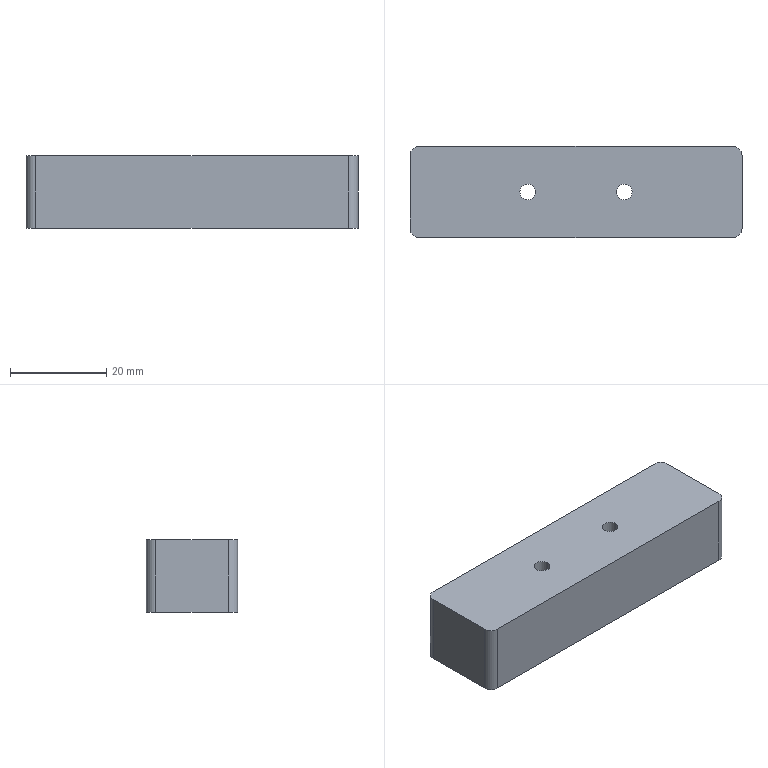Part | STEP file | XL-003 | 1 solid | 20 faces | box 69 x 19 x 15 mm | volume 19058 mm3 | cylinder 12 | plane 8 | commonest cylinder face diameters 3.3 x4 4 x4 7 x4
STEP:
#1=CARTESIAN_POINT('',(28.,9.5,5.));
#2=VERTEX_POINT('',#1);
#3=CARTESIAN_POINT('',(21.,9.5,5.));
#4=VERTEX_POINT('',#3);
#5=CARTESIAN_POINT('',(24.5,9.5,5.));
#6=DIRECTION('',(0.,0.,-1.));
#7=DIRECTION('',(-1.,0.,0.));
#8=AXIS2_PLACEMENT_3D('',#5,#6,#7);
#9=CIRCLE('',#8,3.5);
#10=EDGE_CURVE('',#2,#4,#9,.T.);
#11=ORIENTED_EDGE('',*,*,#10,.F.);
#12=CARTESIAN_POINT('',(28.,9.5,0.));
#13=VERTEX_POINT('',#12);
#14=CARTESIAN_POINT('',(28.,9.5,5.));
#15=DIRECTION('',(0.,0.,-1.));
#16=VECTOR('',#15,1000.);
#17=LINE('',#14,#16);
#18=EDGE_CURVE('',#2,#13,#17,.T.);
#19=ORIENTED_EDGE('',*,*,#18,.T.);
#20=CARTESIAN_POINT('',(21.,9.5,0.));
#21=VERTEX_POINT('',#20);
#22=CARTESIAN_POINT('',(24.5,9.5,0.));
#23=DIRECTION('',(0.,0.,-1.));
#24=DIRECTION('',(-1.,0.,0.));
#25=AXIS2_PLACEMENT_3D('',#22,#23,#24);
#26=CIRCLE('',#25,3.5);
#27=EDGE_CURVE('',#13,#21,#26,.T.);
#28=ORIENTED_EDGE('',*,*,#27,.T.);
#29=CARTESIAN_POINT('',(21.,9.5,5.));
#30=DIRECTION('',(0.,0.,-1.));
#31=VECTOR('',#30,1000.);
#32=LINE('',#29,#31);
#33=EDGE_CURVE('',#4,#21,#32,.T.);
#34=ORIENTED_EDGE('',*,*,#33,.F.);
#35=EDGE_LOOP('',(#11,#19,#28,#34));
#36=FACE_OUTER_BOUND('',#35,.T.);
#37=CARTESIAN_POINT('',(24.5,9.5,5.));
#38=DIRECTION('',(0.,0.,-1.));
#39=DIRECTION('',(-1.,0.,0.));
#40=AXIS2_PLACEMENT_3D('',#37,#38,#39);
#41=CYLINDRICAL_SURFACE('',#40,3.5);
#42=ADVANCED_FACE('',(#36),#41,.F.);
#43=CARTESIAN_POINT('',(48.,9.5,5.));
#44=VERTEX_POINT('',#43);
#45=CARTESIAN_POINT('',(41.,9.5,5.));
#46=VERTEX_POINT('',#45);
#47=CARTESIAN_POINT('',(44.5,9.5,5.));
#48=DIRECTION('',(0.,0.,-1.));
#49=DIRECTION('',(-1.,0.,0.));
#50=AXIS2_PLACEMENT_3D('',#47,#48,#49);
#51=CIRCLE('',#50,3.5);
#52=EDGE_CURVE('',#44,#46,#51,.T.);
#53=ORIENTED_EDGE('',*,*,#52,.F.);
#54=CARTESIAN_POINT('',(48.,9.5,0.));
#55=VERTEX_POINT('',#54);
#56=CARTESIAN_POINT('',(48.,9.5,5.));
#57=DIRECTION('',(0.,0.,-1.));
#58=VECTOR('',#57,1000.);
#59=LINE('',#56,#58);
#60=EDGE_CURVE('',#44,#55,#59,.T.);
#61=ORIENTED_EDGE('',*,*,#60,.T.);
#62=CARTESIAN_POINT('',(41.,9.5,0.));
#63=VERTEX_POINT('',#62);
#64=CARTESIAN_POINT('',(44.5,9.5,0.));
#65=DIRECTION('',(0.,0.,-1.));
#66=DIRECTION('',(-1.,0.,0.));
#67=AXIS2_PLACEMENT_3D('',#64,#65,#66);
#68=CIRCLE('',#67,3.5);
#69=EDGE_CURVE('',#55,#63,#68,.T.);
#70=ORIENTED_EDGE('',*,*,#69,.T.);
#71=CARTESIAN_POINT('',(41.,9.5,5.));
#72=DIRECTION('',(0.,0.,-1.));
#73=VECTOR('',#72,1000.);
#74=LINE('',#71,#73);
#75=EDGE_CURVE('',#46,#63,#74,.T.);
#76=ORIENTED_EDGE('',*,*,#75,.F.);
#77=EDGE_LOOP('',(#53,#61,#70,#76));
#78=FACE_OUTER_BOUND('',#77,.T.);
#79=CARTESIAN_POINT('',(44.5,9.5,5.));
#80=DIRECTION('',(0.,0.,-1.));
#81=DIRECTION('',(-1.,0.,0.));
#82=AXIS2_PLACEMENT_3D('',#79,#80,#81);
#83=CYLINDRICAL_SURFACE('',#82,3.5);
#84=ADVANCED_FACE('',(#78),#83,.F.);
#85=CARTESIAN_POINT('',(46.15,9.5,15.));
#86=VERTEX_POINT('',#85);
#87=CARTESIAN_POINT('',(42.85,9.5,15.));
#88=VERTEX_POINT('',#87);
#89=CARTESIAN_POINT('',(44.5,9.5,15.));
#90=DIRECTION('',(0.,0.,-1.));
#91=DIRECTION('',(-1.,0.,0.));
#92=AXIS2_PLACEMENT_3D('',#89,#90,#91);
#93=CIRCLE('',#92,1.65);
#94=EDGE_CURVE('',#86,#88,#93,.T.);
#95=ORIENTED_EDGE('',*,*,#94,.F.);
#96=CARTESIAN_POINT('',(46.15,9.5,5.));
#97=VERTEX_POINT('',#96);
#98=CARTESIAN_POINT('',(46.15,9.5,15.));
#99=DIRECTION('',(0.,0.,-1.));
#100=VECTOR('',#99,1000.);
#101=LINE('',#98,#100);
#102=EDGE_CURVE('',#86,#97,#101,.T.);
#103=ORIENTED_EDGE('',*,*,#102,.T.);
#104=CARTESIAN_POINT('',(42.85,9.5,5.));
#105=VERTEX_POINT('',#104);
#106=CARTESIAN_POINT('',(44.5,9.5,5.));
#107=DIRECTION('',(0.,0.,1.));
#108=DIRECTION('',(-1.,0.,0.));
#109=AXIS2_PLACEMENT_3D('',#106,#107,#108);
#110=CIRCLE('',#109,1.65);
#111=EDGE_CURVE('',#105,#97,#110,.T.);
#112=ORIENTED_EDGE('',*,*,#111,.F.);
#113=CARTESIAN_POINT('',(42.85,9.5,15.));
#114=DIRECTION('',(0.,0.,-1.));
#115=VECTOR('',#114,1000.);
#116=LINE('',#113,#115);
#117=EDGE_CURVE('',#88,#105,#116,.T.);
#118=ORIENTED_EDGE('',*,*,#117,.F.);
#119=EDGE_LOOP('',(#95,#103,#112,#118));
#120=FACE_OUTER_BOUND('',#119,.T.);
#121=CARTESIAN_POINT('',(44.5,9.5,15.));
#122=DIRECTION('',(0.,0.,-1.));
#123=DIRECTION('',(-1.,0.,0.));
#124=AXIS2_PLACEMENT_3D('',#121,#122,#123);
#125=CYLINDRICAL_SURFACE('',#124,1.65);
#126=ADVANCED_FACE('',(#120),#125,.F.);
#127=CARTESIAN_POINT('',(26.15,9.5,15.));
#128=VERTEX_POINT('',#127);
#129=CARTESIAN_POINT('',(22.85,9.5,15.));
#130=VERTEX_POINT('',#129);
#131=CARTESIAN_POINT('',(24.5,9.5,15.));
#132=DIRECTION('',(0.,0.,-1.));
#133=DIRECTION('',(-1.,0.,0.));
#134=AXIS2_PLACEMENT_3D('',#131,#132,#133);
#135=CIRCLE('',#134,1.65);
#136=EDGE_CURVE('',#128,#130,#135,.T.);
#137=ORIENTED_EDGE('',*,*,#136,.F.);
#138=CARTESIAN_POINT('',(26.15,9.5,5.));
#139=VERTEX_POINT('',#138);
#140=CARTESIAN_POINT('',(26.15,9.5,15.));
#141=DIRECTION('',(0.,0.,-1.));
#142=VECTOR('',#141,1000.);
#143=LINE('',#140,#142);
#144=EDGE_CURVE('',#128,#139,#143,.T.);
#145=ORIENTED_EDGE('',*,*,#144,.T.);
#146=CARTESIAN_POINT('',(22.85,9.5,5.));
#147=VERTEX_POINT('',#146);
#148=CARTESIAN_POINT('',(24.5,9.5,5.));
#149=DIRECTION('',(0.,0.,1.));
#150=DIRECTION('',(-1.,0.,0.));
#151=AXIS2_PLACEMENT_3D('',#148,#149,#150);
#152=CIRCLE('',#151,1.65);
#153=EDGE_CURVE('',#147,#139,#152,.T.);
#154=ORIENTED_EDGE('',*,*,#153,.F.);
#155=CARTESIAN_POINT('',(22.85,9.5,15.));
#156=DIRECTION('',(0.,0.,-1.));
#157=VECTOR('',#156,1000.);
#158=LINE('',#155,#157);
#159=EDGE_CURVE('',#130,#147,#158,.T.);
#160=ORIENTED_EDGE('',*,*,#159,.F.);
#161=EDGE_LOOP('',(#137,#145,#154,#160));
#162=FACE_OUTER_BOUND('',#161,.T.);
#163=CARTESIAN_POINT('',(24.5,9.5,15.));
#164=DIRECTION('',(0.,0.,-1.));
#165=DIRECTION('',(-1.,0.,0.));
#166=AXIS2_PLACEMENT_3D('',#163,#164,#165);
#167=CYLINDRICAL_SURFACE('',#166,1.65);
#168=ADVANCED_FACE('',(#162),#167,.F.);
#169=ORIENTED_EDGE('',*,*,#144,.F.);
#170=CARTESIAN_POINT('',(24.5,9.5,15.));
#171=DIRECTION('',(0.,0.,-1.));
#172=DIRECTION('',(-1.,0.,0.));
#173=AXIS2_PLACEMENT_3D('',#170,#171,#172);
#174=CIRCLE('',#173,1.65);
#175=EDGE_CURVE('',#130,#128,#174,.T.);
#176=ORIENTED_EDGE('',*,*,#175,.F.);
#177=ORIENTED_EDGE('',*,*,#159,.T.);
#178=CARTESIAN_POINT('',(24.5,9.5,5.));
#179=DIRECTION('',(0.,0.,1.));
#180=DIRECTION('',(-1.,0.,0.));
#181=AXIS2_PLACEMENT_3D('',#178,#179,#180);
#182=CIRCLE('',#181,1.65);
#183=EDGE_CURVE('',#139,#147,#182,.T.);
#184=ORIENTED_EDGE('',*,*,#183,.F.);
#185=EDGE_LOOP('',(#169,#176,#177,#184));
#186=FACE_OUTER_BOUND('',#185,.T.);
#187=CARTESIAN_POINT('',(24.5,9.5,15.));
#188=DIRECTION('',(0.,0.,-1.));
#189=DIRECTION('',(-1.,0.,0.));
#190=AXIS2_PLACEMENT_3D('',#187,#188,#189);
#191=CYLINDRICAL_SURFACE('',#190,1.65);
#192=ADVANCED_FACE('',(#186),#191,.F.);
#193=ORIENTED_EDGE('',*,*,#102,.F.);
#194=CARTESIAN_POINT('',(44.5,9.5,15.));
#195=DIRECTION('',(0.,0.,-1.));
#196=DIRECTION('',(-1.,0.,0.));
#197=AXIS2_PLACEMENT_3D('',#194,#195,#196);
#198=CIRCLE('',#197,1.65);
#199=EDGE_CURVE('',#88,#86,#198,.T.);
#200=ORIENTED_EDGE('',*,*,#199,.F.);
#201=ORIENTED_EDGE('',*,*,#117,.T.);
#202=CARTESIAN_POINT('',(44.5,9.5,5.));
#203=DIRECTION('',(0.,0.,1.));
#204=DIRECTION('',(-1.,0.,0.));
#205=AXIS2_PLACEMENT_3D('',#202,#203,#204);
#206=CIRCLE('',#205,1.65);
#207=EDGE_CURVE('',#97,#105,#206,.T.);
#208=ORIENTED_EDGE('',*,*,#207,.F.);
#209=EDGE_LOOP('',(#193,#200,#201,#208));
#210=FACE_OUTER_BOUND('',#209,.T.);
#211=CARTESIAN_POINT('',(44.5,9.5,15.));
#212=DIRECTION('',(0.,0.,-1.));
#213=DIRECTION('',(-1.,0.,0.));
#214=AXIS2_PLACEMENT_3D('',#211,#212,#213);
#215=CYLINDRICAL_SURFACE('',#214,1.65);
#216=ADVANCED_FACE('',(#210),#215,.F.);
#217=CARTESIAN_POINT('',(67.,0.,0.));
#218=VERTEX_POINT('',#217);
#219=CARTESIAN_POINT('',(69.,2.,0.));
#220=VERTEX_POINT('',#219);
#221=CARTESIAN_POINT('',(67.,2.,0.));
#222=DIRECTION('',(0.,0.,1.));
#223=DIRECTION('',(1.,0.,0.));
#224=AXIS2_PLACEMENT_3D('',#221,#222,#223);
#225=CIRCLE('',#224,2.);
#226=EDGE_CURVE('',#218,#220,#225,.T.);
#227=ORIENTED_EDGE('',*,*,#226,.T.);
#228=CARTESIAN_POINT('',(69.,2.,15.));
#229=VERTEX_POINT('',#228);
#230=CARTESIAN_POINT('',(69.,2.,15.));
#231=DIRECTION('',(0.,0.,-1.));
#232=VECTOR('',#231,1000.);
#233=LINE('',#230,#232);
#234=EDGE_CURVE('',#229,#220,#233,.T.);
#235=ORIENTED_EDGE('',*,*,#234,.F.);
#236=CARTESIAN_POINT('',(67.,0.,15.));
#237=VERTEX_POINT('',#236);
#238=CARTESIAN_POINT('',(67.,2.,15.));
#239=DIRECTION('',(0.,0.,1.));
#240=DIRECTION('',(1.,0.,0.));
#241=AXIS2_PLACEMENT_3D('',#238,#239,#240);
#242=CIRCLE('',#241,2.);
#243=EDGE_CURVE('',#237,#229,#242,.T.);
#244=ORIENTED_EDGE('',*,*,#243,.F.);
#245=CARTESIAN_POINT('',(67.,0.,15.));
#246=DIRECTION('',(0.,0.,-1.));
#247=VECTOR('',#246,1000.);
#248=LINE('',#245,#247);
#249=EDGE_CURVE('',#237,#218,#248,.T.);
#250=ORIENTED_EDGE('',*,*,#249,.T.);
#251=EDGE_LOOP('',(#227,#235,#244,#250));
#252=FACE_OUTER_BOUND('',#251,.T.);
#253=CARTESIAN_POINT('',(67.,2.,15.));
#254=DIRECTION('',(0.,0.,-1.));
#255=DIRECTION('',(-1.,0.,0.));
#256=AXIS2_PLACEMENT_3D('',#253,#254,#255);
#257=CYLINDRICAL_SURFACE('',#256,2.);
#258=ADVANCED_FACE('',(#252),#257,.T.);
#259=CARTESIAN_POINT('',(69.,17.,0.));
#260=VERTEX_POINT('',#259);
#261=CARTESIAN_POINT('',(69.,2.,0.));
#262=DIRECTION('',(0.,1.,0.));
#263=VECTOR('',#262,1000.);
#264=LINE('',#261,#263);
#265=EDGE_CURVE('',#220,#260,#264,.T.);
#266=ORIENTED_EDGE('',*,*,#265,.T.);
#267=CARTESIAN_POINT('',(69.,17.,15.));
#268=VERTEX_POINT('',#267);
#269=CARTESIAN_POINT('',(69.,17.,15.));
#270=DIRECTION('',(0.,0.,-1.));
#271=VECTOR('',#270,1000.);
#272=LINE('',#269,#271);
#273=EDGE_CURVE('',#268,#260,#272,.T.);
#274=ORIENTED_EDGE('',*,*,#273,.F.);
#275=CARTESIAN_POINT('',(69.,2.,15.));
#276=DIRECTION('',(0.,1.,0.));
#277=VECTOR('',#276,1000.);
#278=LINE('',#275,#277);
#279=EDGE_CURVE('',#229,#268,#278,.T.);
#280=ORIENTED_EDGE('',*,*,#279,.F.);
#281=ORIENTED_EDGE('',*,*,#234,.T.);
#282=EDGE_LOOP('',(#266,#274,#280,#281));
#283=FACE_OUTER_BOUND('',#282,.T.);
#284=CARTESIAN_POINT('',(69.,2.,15.));
#285=DIRECTION('',(-1.,0.,0.));
#286=DIRECTION('',(0.,0.,1.));
#287=AXIS2_PLACEMENT_3D('',#284,#285,#286);
#288=PLANE('',#287);
#289=ADVANCED_FACE('',(#283),#288,.F.);
#290=CARTESIAN_POINT('',(67.,19.,0.));
#291=VERTEX_POINT('',#290);
#292=CARTESIAN_POINT('',(67.,17.,0.));
#293=DIRECTION('',(0.,0.,1.));
#294=DIRECTION('',(-1.,0.,0.));
#295=AXIS2_PLACEMENT_3D('',#292,#293,#294);
#296=CIRCLE('',#295,2.);
#297=EDGE_CURVE('',#260,#291,#296,.T.);
#298=ORIENTED_EDGE('',*,*,#297,.T.);
#299=CARTESIAN_POINT('',(67.,19.,15.));
#300=VERTEX_POINT('',#299);
#301=CARTESIAN_POINT('',(67.,19.,15.));
#302=DIRECTION('',(0.,0.,-1.));
#303=VECTOR('',#302,1000.);
#304=LINE('',#301,#303);
#305=EDGE_CURVE('',#300,#291,#304,.T.);
#306=ORIENTED_EDGE('',*,*,#305,.F.);
#307=CARTESIAN_POINT('',(67.,17.,15.));
#308=DIRECTION('',(0.,0.,1.));
#309=DIRECTION('',(-1.,0.,0.));
#310=AXIS2_PLACEMENT_3D('',#307,#308,#309);
#311=CIRCLE('',#310,2.);
#312=EDGE_CURVE('',#268,#300,#311,.T.);
#313=ORIENTED_EDGE('',*,*,#312,.F.);
#314=ORIENTED_EDGE('',*,*,#273,.T.);
#315=EDGE_LOOP('',(#298,#306,#313,#314));
#316=FACE_OUTER_BOUND('',#315,.T.);
#317=CARTESIAN_POINT('',(67.,17.,15.));
#318=DIRECTION('',(0.,0.,-1.));
#319=DIRECTION('',(-1.,0.,0.));
#320=AXIS2_PLACEMENT_3D('',#317,#318,#319);
#321=CYLINDRICAL_SURFACE('',#320,2.);
#322=ADVANCED_FACE('',(#316),#321,.T.);
#323=CARTESIAN_POINT('',(2.,19.,0.));
#324=VERTEX_POINT('',#323);
#325=CARTESIAN_POINT('',(2.,19.,0.));
#326=DIRECTION('',(-1.,0.,0.));
#327=VECTOR('',#326,1000.);
#328=LINE('',#325,#327);
#329=EDGE_CURVE('',#291,#324,#328,.T.);
#330=ORIENTED_EDGE('',*,*,#329,.T.);
#331=CARTESIAN_POINT('',(2.,19.,15.));
#332=VERTEX_POINT('',#331);
#333=CARTESIAN_POINT('',(2.,19.,15.));
#334=DIRECTION('',(0.,0.,-1.));
#335=VECTOR('',#334,1000.);
#336=LINE('',#333,#335);
#337=EDGE_CURVE('',#332,#324,#336,.T.);
#338=ORIENTED_EDGE('',*,*,#337,.F.);
#339=CARTESIAN_POINT('',(2.,19.,15.));
#340=DIRECTION('',(-1.,0.,0.));
#341=VECTOR('',#340,1000.);
#342=LINE('',#339,#341);
#343=EDGE_CURVE('',#300,#332,#342,.T.);
#344=ORIENTED_EDGE('',*,*,#343,.F.);
#345=ORIENTED_EDGE('',*,*,#305,.T.);
#346=EDGE_LOOP('',(#330,#338,#344,#345));
#347=FACE_OUTER_BOUND('',#346,.T.);
#348=CARTESIAN_POINT('',(2.,19.,15.));
#349=DIRECTION('',(0.,-1.,0.));
#350=DIRECTION('',(0.,0.,-1.));
#351=AXIS2_PLACEMENT_3D('',#348,#349,#350);
#352=PLANE('',#351);
#353=ADVANCED_FACE('',(#347),#352,.F.);
#354=CARTESIAN_POINT('',(0.,17.,0.));
#355=VERTEX_POINT('',#354);
#356=CARTESIAN_POINT('',(2.,17.,0.));
#357=DIRECTION('',(0.,0.,1.));
#358=DIRECTION('',(-1.,0.,0.));
#359=AXIS2_PLACEMENT_3D('',#356,#357,#358);
#360=CIRCLE('',#359,2.);
#361=EDGE_CURVE('',#324,#355,#360,.T.);
#362=ORIENTED_EDGE('',*,*,#361,.T.);
#363=CARTESIAN_POINT('',(0.,17.,15.));
#364=VERTEX_POINT('',#363);
#365=CARTESIAN_POINT('',(0.,17.,15.));
#366=DIRECTION('',(0.,0.,-1.));
#367=VECTOR('',#366,1000.);
#368=LINE('',#365,#367);
#369=EDGE_CURVE('',#364,#355,#368,.T.);
#370=ORIENTED_EDGE('',*,*,#369,.F.);
#371=CARTESIAN_POINT('',(2.,17.,15.));
#372=DIRECTION('',(0.,0.,1.));
#373=DIRECTION('',(-1.,0.,0.));
#374=AXIS2_PLACEMENT_3D('',#371,#372,#373);
#375=CIRCLE('',#374,2.);
#376=EDGE_CURVE('',#332,#364,#375,.T.);
#377=ORIENTED_EDGE('',*,*,#376,.F.);
#378=ORIENTED_EDGE('',*,*,#337,.T.);
#379=EDGE_LOOP('',(#362,#370,#377,#378));
#380=FACE_OUTER_BOUND('',#379,.T.);
#381=CARTESIAN_POINT('',(2.,17.,15.));
#382=DIRECTION('',(0.,0.,-1.));
#383=DIRECTION('',(-1.,0.,0.));
#384=AXIS2_PLACEMENT_3D('',#381,#382,#383);
#385=CYLINDRICAL_SURFACE('',#384,2.);
#386=ADVANCED_FACE('',(#380),#385,.T.);
#387=CARTESIAN_POINT('',(0.,2.,0.));
#388=VERTEX_POINT('',#387);
#389=CARTESIAN_POINT('',(0.,2.,0.));
#390=DIRECTION('',(0.,-1.,0.));
#391=VECTOR('',#390,1000.);
#392=LINE('',#389,#391);
#393=EDGE_CURVE('',#355,#388,#392,.T.);
#394=ORIENTED_EDGE('',*,*,#393,.T.);
#395=CARTESIAN_POINT('',(0.,2.,15.));
#396=VERTEX_POINT('',#395);
#397=CARTESIAN_POINT('',(0.,2.,15.));
#398=DIRECTION('',(0.,0.,-1.));
#399=VECTOR('',#398,1000.);
#400=LINE('',#397,#399);
#401=EDGE_CURVE('',#396,#388,#400,.T.);
#402=ORIENTED_EDGE('',*,*,#401,.F.);
#403=CARTESIAN_POINT('',(0.,2.,15.));
#404=DIRECTION('',(0.,-1.,0.));
#405=VECTOR('',#404,1000.);
#406=LINE('',#403,#405);
#407=EDGE_CURVE('',#364,#396,#406,.T.);
#408=ORIENTED_EDGE('',*,*,#407,.F.);
#409=ORIENTED_EDGE('',*,*,#369,.T.);
#410=EDGE_LOOP('',(#394,#402,#408,#409));
#411=FACE_OUTER_BOUND('',#410,.T.);
#412=CARTESIAN_POINT('',(0.,2.,15.));
#413=DIRECTION('',(1.,0.,0.));
#414=DIRECTION('',(0.,0.,-1.));
#415=AXIS2_PLACEMENT_3D('',#412,#413,#414);
#416=PLANE('',#415);
#417=ADVANCED_FACE('',(#411),#416,.F.);
#418=CARTESIAN_POINT('',(2.,0.,0.));
#419=VERTEX_POINT('',#418);
#420=CARTESIAN_POINT('',(2.,2.,0.));
#421=DIRECTION('',(0.,0.,1.));
#422=DIRECTION('',(-1.,0.,0.));
#423=AXIS2_PLACEMENT_3D('',#420,#421,#422);
#424=CIRCLE('',#423,2.);
#425=EDGE_CURVE('',#388,#419,#424,.T.);
#426=ORIENTED_EDGE('',*,*,#425,.T.);
#427=CARTESIAN_POINT('',(2.,0.,15.));
#428=VERTEX_POINT('',#427);
#429=CARTESIAN_POINT('',(2.,0.,15.));
#430=DIRECTION('',(0.,0.,-1.));
#431=VECTOR('',#430,1000.);
#432=LINE('',#429,#431);
#433=EDGE_CURVE('',#428,#419,#432,.T.);
#434=ORIENTED_EDGE('',*,*,#433,.F.);
#435=CARTESIAN_POINT('',(2.,2.,15.));
#436=DIRECTION('',(0.,0.,1.));
#437=DIRECTION('',(-1.,0.,0.));
#438=AXIS2_PLACEMENT_3D('',#435,#436,#437);
#439=CIRCLE('',#438,2.);
#440=EDGE_CURVE('',#396,#428,#439,.T.);
#441=ORIENTED_EDGE('',*,*,#440,.F.);
#442=ORIENTED_EDGE('',*,*,#401,.T.);
#443=EDGE_LOOP('',(#426,#434,#441,#442));
#444=FACE_OUTER_BOUND('',#443,.T.);
#445=CARTESIAN_POINT('',(2.,2.,15.));
#446=DIRECTION('',(0.,0.,-1.));
#447=DIRECTION('',(-1.,0.,0.));
#448=AXIS2_PLACEMENT_3D('',#445,#446,#447);
#449=CYLINDRICAL_SURFACE('',#448,2.);
#450=ADVANCED_FACE('',(#444),#449,.T.);
#451=CARTESIAN_POINT('',(2.,0.,0.));
#452=DIRECTION('',(1.,0.,0.));
#453=VECTOR('',#452,1000.);
#454=LINE('',#451,#453);
#455=EDGE_CURVE('',#419,#218,#454,.T.);
#456=ORIENTED_EDGE('',*,*,#455,.T.);
#457=ORIENTED_EDGE('',*,*,#249,.F.);
#458=CARTESIAN_POINT('',(2.,0.,15.));
#459=DIRECTION('',(1.,0.,0.));
#460=VECTOR('',#459,1000.);
#461=LINE('',#458,#460);
#462=EDGE_CURVE('',#428,#237,#461,.T.);
#463=ORIENTED_EDGE('',*,*,#462,.F.);
#464=ORIENTED_EDGE('',*,*,#433,.T.);
#465=EDGE_LOOP('',(#456,#457,#463,#464));
#466=FACE_OUTER_BOUND('',#465,.T.);
#467=CARTESIAN_POINT('',(2.,0.,15.));
#468=DIRECTION('',(0.,1.,0.));
#469=DIRECTION('',(0.,0.,1.));
#470=AXIS2_PLACEMENT_3D('',#467,#468,#469);
#471=PLANE('',#470);
#472=ADVANCED_FACE('',(#466),#471,.F.);
#473=ORIENTED_EDGE('',*,*,#199,.T.);
#474=ORIENTED_EDGE('',*,*,#94,.T.);
#475=EDGE_LOOP('',(#473,#474));
#476=FACE_BOUND('',#475,.T.);
#477=ORIENTED_EDGE('',*,*,#175,.T.);
#478=ORIENTED_EDGE('',*,*,#136,.T.);
#479=EDGE_LOOP('',(#477,#478));
#480=FACE_BOUND('',#479,.T.);
#481=ORIENTED_EDGE('',*,*,#243,.T.);
#482=ORIENTED_EDGE('',*,*,#279,.T.);
#483=ORIENTED_EDGE('',*,*,#312,.T.);
#484=ORIENTED_EDGE('',*,*,#343,.T.);
#485=ORIENTED_EDGE('',*,*,#376,.T.);
#486=ORIENTED_EDGE('',*,*,#407,.T.);
#487=ORIENTED_EDGE('',*,*,#440,.T.);
#488=ORIENTED_EDGE('',*,*,#462,.T.);
#489=EDGE_LOOP('',(#481,#482,#483,#484,#485,#486,#487,#488));
#490=FACE_OUTER_BOUND('',#489,.T.);
#491=CARTESIAN_POINT('',(67.,2.,15.));
#492=DIRECTION('',(0.,0.,1.));
#493=DIRECTION('',(1.,0.,0.));
#494=AXIS2_PLACEMENT_3D('',#491,#492,#493);
#495=PLANE('',#494);
#496=ADVANCED_FACE('',(#476,#480,#490),#495,.T.);
#497=CARTESIAN_POINT('',(44.5,9.5,0.));
#498=DIRECTION('',(0.,0.,-1.));
#499=DIRECTION('',(-1.,0.,0.));
#500=AXIS2_PLACEMENT_3D('',#497,#498,#499);
#501=CIRCLE('',#500,3.5);
#502=EDGE_CURVE('',#63,#55,#501,.T.);
#503=ORIENTED_EDGE('',*,*,#502,.F.);
#504=ORIENTED_EDGE('',*,*,#69,.F.);
#505=EDGE_LOOP('',(#503,#504));
#506=FACE_BOUND('',#505,.T.);
#507=CARTESIAN_POINT('',(24.5,9.5,0.));
#508=DIRECTION('',(0.,0.,-1.));
#509=DIRECTION('',(-1.,0.,0.));
#510=AXIS2_PLACEMENT_3D('',#507,#508,#509);
#511=CIRCLE('',#510,3.5);
#512=EDGE_CURVE('',#21,#13,#511,.T.);
#513=ORIENTED_EDGE('',*,*,#512,.F.);
#514=ORIENTED_EDGE('',*,*,#27,.F.);
#515=EDGE_LOOP('',(#513,#514));
#516=FACE_BOUND('',#515,.T.);
#517=ORIENTED_EDGE('',*,*,#226,.F.);
#518=ORIENTED_EDGE('',*,*,#455,.F.);
#519=ORIENTED_EDGE('',*,*,#425,.F.);
#520=ORIENTED_EDGE('',*,*,#393,.F.);
#521=ORIENTED_EDGE('',*,*,#361,.F.);
#522=ORIENTED_EDGE('',*,*,#329,.F.);
#523=ORIENTED_EDGE('',*,*,#297,.F.);
#524=ORIENTED_EDGE('',*,*,#265,.F.);
#525=EDGE_LOOP('',(#517,#518,#519,#520,#521,#522,#523,#524));
#526=FACE_OUTER_BOUND('',#525,.T.);
#527=CARTESIAN_POINT('',(67.,2.,0.));
#528=DIRECTION('',(0.,0.,1.));
#529=DIRECTION('',(1.,0.,0.));
#530=AXIS2_PLACEMENT_3D('',#527,#528,#529);
#531=PLANE('',#530);
#532=ADVANCED_FACE('',(#506,#516,#526),#531,.F.);
#533=CARTESIAN_POINT('',(44.5,9.5,5.));
#534=DIRECTION('',(0.,0.,-1.));
#535=DIRECTION('',(-1.,0.,0.));
#536=AXIS2_PLACEMENT_3D('',#533,#534,#535);
#537=CIRCLE('',#536,3.5);
#538=EDGE_CURVE('',#46,#44,#537,.T.);
#539=ORIENTED_EDGE('',*,*,#538,.T.);
#540=ORIENTED_EDGE('',*,*,#52,.T.);
#541=EDGE_LOOP('',(#539,#540));
#542=FACE_OUTER_BOUND('',#541,.T.);
#543=ORIENTED_EDGE('',*,*,#111,.T.);
#544=ORIENTED_EDGE('',*,*,#207,.T.);
#545=EDGE_LOOP('',(#543,#544));
#546=FACE_BOUND('',#545,.T.);
#547=CARTESIAN_POINT('',(44.5,9.5,5.));
#548=DIRECTION('',(0.,0.,-1.));
#549=DIRECTION('',(-1.,0.,0.));
#550=AXIS2_PLACEMENT_3D('',#547,#548,#549);
#551=PLANE('',#550);
#552=ADVANCED_FACE('',(#542,#546),#551,.T.);
#553=ORIENTED_EDGE('',*,*,#60,.F.);
#554=ORIENTED_EDGE('',*,*,#538,.F.);
#555=ORIENTED_EDGE('',*,*,#75,.T.);
#556=ORIENTED_EDGE('',*,*,#502,.T.);
#557=EDGE_LOOP('',(#553,#554,#555,#556));
#558=FACE_OUTER_BOUND('',#557,.T.);
#559=CARTESIAN_POINT('',(44.5,9.5,5.));
#560=DIRECTION('',(0.,0.,-1.));
#561=DIRECTION('',(-1.,0.,0.));
#562=AXIS2_PLACEMENT_3D('',#559,#560,#561);
#563=CYLINDRICAL_SURFACE('',#562,3.5);
#564=ADVANCED_FACE('',(#558),#563,.F.);
#565=CARTESIAN_POINT('',(24.5,9.5,5.));
#566=DIRECTION('',(0.,0.,-1.));
#567=DIRECTION('',(-1.,0.,0.));
#568=AXIS2_PLACEMENT_3D('',#565,#566,#567);
#569=CIRCLE('',#568,3.5);
#570=EDGE_CURVE('',#4,#2,#569,.T.);
#571=ORIENTED_EDGE('',*,*,#570,.T.);
#572=ORIENTED_EDGE('',*,*,#10,.T.);
#573=EDGE_LOOP('',(#571,#572));
#574=FACE_OUTER_BOUND('',#573,.T.);
#575=ORIENTED_EDGE('',*,*,#153,.T.);
#576=ORIENTED_EDGE('',*,*,#183,.T.);
#577=EDGE_LOOP('',(#575,#576));
#578=FACE_BOUND('',#577,.T.);
#579=CARTESIAN_POINT('',(24.5,9.5,5.));
#580=DIRECTION('',(0.,0.,-1.));
#581=DIRECTION('',(-1.,0.,0.));
#582=AXIS2_PLACEMENT_3D('',#579,#580,#581);
#583=PLANE('',#582);
#584=ADVANCED_FACE('',(#574,#578),#583,.T.);
#585=ORIENTED_EDGE('',*,*,#18,.F.);
#586=ORIENTED_EDGE('',*,*,#570,.F.);
#587=ORIENTED_EDGE('',*,*,#33,.T.);
#588=ORIENTED_EDGE('',*,*,#512,.T.);
#589=EDGE_LOOP('',(#585,#586,#587,#588));
#590=FACE_OUTER_BOUND('',#589,.T.);
#591=CARTESIAN_POINT('',(24.5,9.5,5.));
#592=DIRECTION('',(0.,0.,-1.));
#593=DIRECTION('',(-1.,0.,0.));
#594=AXIS2_PLACEMENT_3D('',#591,#592,#593);
#595=CYLINDRICAL_SURFACE('',#594,3.5);
#596=ADVANCED_FACE('',(#590),#595,.F.);
#597=CLOSED_SHELL('',(#42,#84,#126,#168,#192,#216,#258,#289,#322,#353,#386,#417,#450,#472,#496,#532,#552,#564,#584,#596));
#598=MANIFOLD_SOLID_BREP('',#597);
#599=CARTESIAN_POINT('',(0.,0.,0.));
#600=DIRECTION('',(0.,0.,1.));
#601=DIRECTION('',(1.,0.,0.));
#602=AXIS2_PLACEMENT_3D('',#599,#600,#601);
#603=(LENGTH_UNIT()NAMED_UNIT(*)SI_UNIT(.MILLI.,.METRE.));
#604=UNCERTAINTY_MEASURE_WITH_UNIT(LENGTH_MEASURE(0.00001),#603,'','');
#605=(NAMED_UNIT(*)PLANE_ANGLE_UNIT()SI_UNIT($,.RADIAN.));
#606=(NAMED_UNIT(*)SI_UNIT($,.STERADIAN.)SOLID_ANGLE_UNIT());
#607=(GEOMETRIC_REPRESENTATION_CONTEXT(3)GLOBAL_UNCERTAINTY_ASSIGNED_CONTEXT((#604))GLOBAL_UNIT_ASSIGNED_CONTEXT((#603,#605,#606))REPRESENTATION_CONTEXT('',''));
#608=ADVANCED_BREP_SHAPE_REPRESENTATION('',(#598,#602),#607);